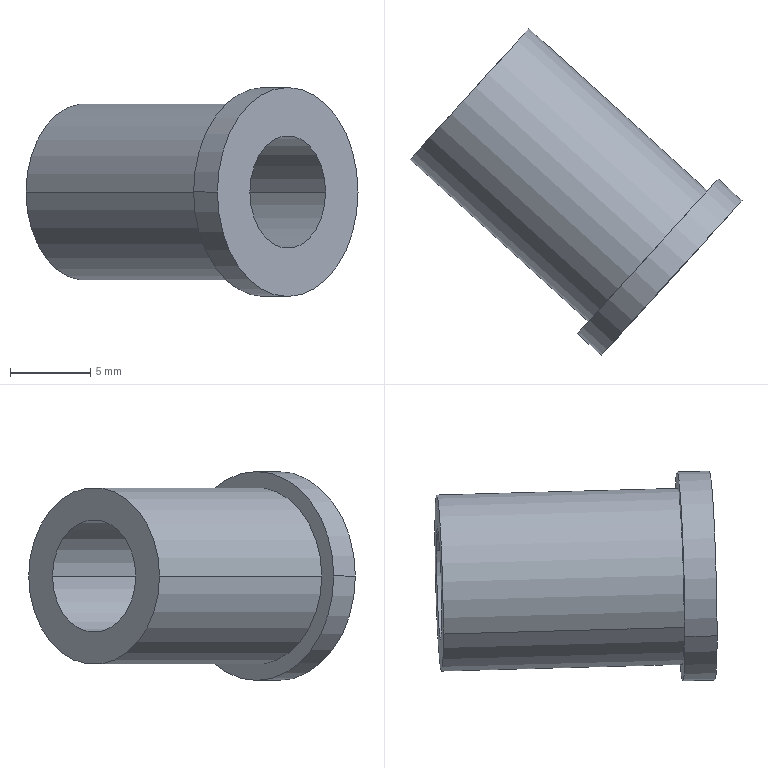Part | STEP file | PRT0001_68_29 | 1 solid | 9 faces | box 20.651 x 20.315 x 13 mm | volume 1037 mm3 | cylinder 6 | plane 3 | commonest cylinder face diameters 7 x2 11 x2 13 x2
STEP:
#1=CARTESIAN_POINT('',(0.,0.,0.));
#2=DIRECTION('',(0.,0.,1.));
#3=DIRECTION('',(1.,0.,0.));
#4=AXIS2_PLACEMENT_3D('',#1,#2,#3);
#5=CARTESIAN_POINT('',(1767.354,865.18,0.000000606));
#6=VERTEX_POINT('',#5);
#7=CARTESIAN_POINT('',(1774.754,873.318,0.000000606));
#8=VERTEX_POINT('',#7);
#9=CARTESIAN_POINT('',(1771.054,869.249,0.000000606));
#10=DIRECTION('',(0.7399,-0.6727,0.));
#11=DIRECTION('',(-0.6727,-0.7399,0.));
#12=AXIS2_PLACEMENT_3D('',#9,#10,#11);
#13=CIRCLE('',#12,5.5);
#14=CARTESIAN_POINT('',(536.884,-488.145,-24.));
#15=DIRECTION('',(-0.7399,0.6727,0.));
#16=DIRECTION('',(0.6727,0.7399,0.));
#17=AXIS2_PLACEMENT_3D('',#14,#15,#16);
#18=PLANE('',#17);
#19=CARTESIAN_POINT('',(1829.083,-24.));
#20=CARTESIAN_POINT('',(1829.083,-14.474));
#21=CARTESIAN_POINT('',(1837.333,-19.237));
#22=CARTESIAN_POINT('',(1845.583,-24.));
#23=CARTESIAN_POINT('',(1837.333,-28.763));
#24=CARTESIAN_POINT('',(1829.083,-33.526));
#25=CARTESIAN_POINT('',(1829.083,-24.));
#26=(BOUNDED_CURVE()B_SPLINE_CURVE(2,(#19,#20,#21,#22,#23,#24,#25),.UNSPECIFIED.,.T.,.F.)B_SPLINE_CURVE_WITH_KNOTS((1,2,2,2,2,1),(-2.094,0.,2.094,4.189,6.283,8.378),.UNSPECIFIED.)CURVE()GEOMETRIC_REPRESENTATION_ITEM()RATIONAL_B_SPLINE_CURVE((1.,0.5,1.,0.5,1.,0.5,1.))REPRESENTATION_ITEM(''));
#27=(GEOMETRIC_REPRESENTATION_CONTEXT(2)PARAMETRIC_REPRESENTATION_CONTEXT()REPRESENTATION_CONTEXT('',''));
#28=DEFINITIONAL_REPRESENTATION('',(#26),#27);
#29=PCURVE('',#18,#28);
#30=CARTESIAN_POINT('',(1780.673,860.504,0.000000606));
#31=DIRECTION('',(-0.7399,0.6727,0.));
#32=DIRECTION('',(0.6727,0.7399,0.));
#33=AXIS2_PLACEMENT_3D('',#30,#31,#32);
#34=CYLINDRICAL_SURFACE('',#33,5.5);
#35=CARTESIAN_POINT('',(3.142,13.));
#36=DIRECTION('',(-1.,0.));
#37=VECTOR('',#36,1.);
#38=LINE('',#35,#37);
#39=(GEOMETRIC_REPRESENTATION_CONTEXT(2)PARAMETRIC_REPRESENTATION_CONTEXT()REPRESENTATION_CONTEXT('',''));
#40=DEFINITIONAL_REPRESENTATION('',(#38),#39);
#41=PCURVE('',#34,#40);
#42=SURFACE_CURVE('',#13,(#29,#41),.PCURVE_S1.);
#43=EDGE_CURVE('',#6,#8,#42,.T.);
#44=ORIENTED_EDGE('',*,*,#43,.T.);
#45=CARTESIAN_POINT('',(1771.054,869.249,0.000000606));
#46=DIRECTION('',(0.7399,-0.6727,0.));
#47=DIRECTION('',(0.6727,0.7399,0.));
#48=AXIS2_PLACEMENT_3D('',#45,#46,#47);
#49=CIRCLE('',#48,5.5);
#50=CARTESIAN_POINT('',(1840.083,-24.));
#51=CARTESIAN_POINT('',(1840.083,-33.526));
#52=CARTESIAN_POINT('',(1831.833,-28.763));
#53=CARTESIAN_POINT('',(1823.583,-24.));
#54=CARTESIAN_POINT('',(1831.833,-19.237));
#55=CARTESIAN_POINT('',(1840.083,-14.474));
#56=CARTESIAN_POINT('',(1840.083,-24.));
#57=(BOUNDED_CURVE()B_SPLINE_CURVE(2,(#50,#51,#52,#53,#54,#55,#56),.UNSPECIFIED.,.T.,.F.)B_SPLINE_CURVE_WITH_KNOTS((1,2,2,2,2,1),(-2.094,0.,2.094,4.189,6.283,8.378),.UNSPECIFIED.)CURVE()GEOMETRIC_REPRESENTATION_ITEM()RATIONAL_B_SPLINE_CURVE((1.,0.5,1.,0.5,1.,0.5,1.))REPRESENTATION_ITEM(''));
#58=(GEOMETRIC_REPRESENTATION_CONTEXT(2)PARAMETRIC_REPRESENTATION_CONTEXT()REPRESENTATION_CONTEXT('',''));
#59=DEFINITIONAL_REPRESENTATION('',(#57),#58);
#60=PCURVE('',#18,#59);
#61=CARTESIAN_POINT('',(1780.673,860.504,0.000000606));
#62=DIRECTION('',(-0.7399,0.6727,0.));
#63=DIRECTION('',(0.6727,0.7399,0.));
#64=AXIS2_PLACEMENT_3D('',#61,#62,#63);
#65=CYLINDRICAL_SURFACE('',#64,5.5);
#66=CARTESIAN_POINT('',(6.283,13.));
#67=DIRECTION('',(-1.,0.));
#68=VECTOR('',#67,1.);
#69=LINE('',#66,#68);
#70=(GEOMETRIC_REPRESENTATION_CONTEXT(2)PARAMETRIC_REPRESENTATION_CONTEXT()REPRESENTATION_CONTEXT('',''));
#71=DEFINITIONAL_REPRESENTATION('',(#69),#70);
#72=PCURVE('',#65,#71);
#73=SURFACE_CURVE('',#49,(#60,#72),.PCURVE_S1.);
#74=EDGE_CURVE('',#8,#6,#73,.T.);
#75=ORIENTED_EDGE('',*,*,#74,.T.);
#76=EDGE_LOOP('',(#44,#75));
#77=FACE_BOUND('',#76,.F.);
#78=CARTESIAN_POINT('',(1768.7,866.659,0.000000606));
#79=VERTEX_POINT('',#78);
#80=CARTESIAN_POINT('',(1773.409,871.839,0.000000606));
#81=VERTEX_POINT('',#80);
#82=CARTESIAN_POINT('',(1771.054,869.249,0.000000606));
#83=DIRECTION('',(-0.7399,0.6727,0.));
#84=DIRECTION('',(-0.6727,-0.7399,0.));
#85=AXIS2_PLACEMENT_3D('',#82,#83,#84);
#86=CIRCLE('',#85,3.5);
#87=CARTESIAN_POINT('',(1834.583,-24.));
#88=DIRECTION('',(-1.,0.));
#89=AXIS2_PLACEMENT_2D('',#87,#88);
#90=CIRCLE('',#89,3.5);
#91=(GEOMETRIC_REPRESENTATION_CONTEXT(2)PARAMETRIC_REPRESENTATION_CONTEXT()REPRESENTATION_CONTEXT('',''));
#92=DEFINITIONAL_REPRESENTATION('',(#90),#91);
#93=PCURVE('',#18,#92);
#94=CARTESIAN_POINT('',(1780.673,860.504,0.000000606));
#95=DIRECTION('',(-0.7399,0.6727,0.));
#96=DIRECTION('',(0.6727,0.7399,0.));
#97=AXIS2_PLACEMENT_3D('',#94,#95,#96);
#98=CYLINDRICAL_SURFACE('',#97,3.5);
#99=CARTESIAN_POINT('',(3.142,13.));
#100=DIRECTION('',(1.,0.));
#101=VECTOR('',#100,1.);
#102=LINE('',#99,#101);
#103=(GEOMETRIC_REPRESENTATION_CONTEXT(2)PARAMETRIC_REPRESENTATION_CONTEXT()REPRESENTATION_CONTEXT('',''));
#104=DEFINITIONAL_REPRESENTATION('',(#102),#103);
#105=PCURVE('',#98,#104);
#106=SURFACE_CURVE('',#86,(#93,#105),.PCURVE_S1.);
#107=EDGE_CURVE('',#79,#81,#106,.T.);
#108=ORIENTED_EDGE('',*,*,#107,.T.);
#109=CARTESIAN_POINT('',(1771.054,869.249,0.000000606));
#110=DIRECTION('',(-0.7399,0.6727,0.));
#111=DIRECTION('',(0.6727,0.7399,0.));
#112=AXIS2_PLACEMENT_3D('',#109,#110,#111);
#113=CIRCLE('',#112,3.5);
#114=CARTESIAN_POINT('',(1834.583,-24.));
#115=DIRECTION('',(1.,0.));
#116=AXIS2_PLACEMENT_2D('',#114,#115);
#117=CIRCLE('',#116,3.5);
#118=(GEOMETRIC_REPRESENTATION_CONTEXT(2)PARAMETRIC_REPRESENTATION_CONTEXT()REPRESENTATION_CONTEXT('',''));
#119=DEFINITIONAL_REPRESENTATION('',(#117),#118);
#120=PCURVE('',#18,#119);
#121=CARTESIAN_POINT('',(1780.673,860.504,0.000000606));
#122=DIRECTION('',(-0.7399,0.6727,0.));
#123=DIRECTION('',(0.6727,0.7399,0.));
#124=AXIS2_PLACEMENT_3D('',#121,#122,#123);
#125=CYLINDRICAL_SURFACE('',#124,3.5);
#126=CARTESIAN_POINT('',(0.,13.));
#127=DIRECTION('',(1.,0.));
#128=VECTOR('',#127,1.);
#129=LINE('',#126,#128);
#130=(GEOMETRIC_REPRESENTATION_CONTEXT(2)PARAMETRIC_REPRESENTATION_CONTEXT()REPRESENTATION_CONTEXT('',''));
#131=DEFINITIONAL_REPRESENTATION('',(#129),#130);
#132=PCURVE('',#125,#131);
#133=SURFACE_CURVE('',#113,(#120,#132),.PCURVE_S1.);
#134=EDGE_CURVE('',#81,#79,#133,.T.);
#135=ORIENTED_EDGE('',*,*,#134,.T.);
#136=EDGE_LOOP('',(#108,#135));
#137=FACE_BOUND('',#136,.F.);
#138=ADVANCED_FACE('',(#77,#137),#18,.T.);
#139=CARTESIAN_POINT('',(1778.452,855.089,0.000000606));
#140=VERTEX_POINT('',#139);
#141=CARTESIAN_POINT('',(1767.354,865.18,0.000000606));
#142=DIRECTION('',(0.7399,-0.6727,0.));
#143=VECTOR('',#142,1.);
#144=LINE('',#141,#143);
#145=CARTESIAN_POINT('',(3.142,13.));
#146=DIRECTION('',(0.,-1.));
#147=VECTOR('',#146,1.);
#148=LINE('',#145,#147);
#149=(GEOMETRIC_REPRESENTATION_CONTEXT(2)PARAMETRIC_REPRESENTATION_CONTEXT()REPRESENTATION_CONTEXT('',''));
#150=DEFINITIONAL_REPRESENTATION('',(#148),#149);
#151=PCURVE('',#34,#150);
#152=CARTESIAN_POINT('',(3.142,13.));
#153=DIRECTION('',(0.,-1.));
#154=VECTOR('',#153,1.);
#155=LINE('',#152,#154);
#156=(GEOMETRIC_REPRESENTATION_CONTEXT(2)PARAMETRIC_REPRESENTATION_CONTEXT()REPRESENTATION_CONTEXT('',''));
#157=DEFINITIONAL_REPRESENTATION('',(#155),#156);
#158=PCURVE('',#65,#157);
#159=SURFACE_CURVE('',#144,(#151,#158),.PCURVE_S1.);
#160=EDGE_CURVE('',#6,#140,#159,.T.);
#161=ORIENTED_EDGE('',*,*,#160,.F.);
#162=ORIENTED_EDGE('',*,*,#43,.T.);
#163=CARTESIAN_POINT('',(1785.852,863.228,0.000000606));
#164=VERTEX_POINT('',#163);
#165=CARTESIAN_POINT('',(1774.754,873.318,0.000000606));
#166=DIRECTION('',(0.7399,-0.6727,0.));
#167=VECTOR('',#166,1.);
#168=LINE('',#165,#167);
#169=CARTESIAN_POINT('',(0.,13.));
#170=DIRECTION('',(0.,-1.));
#171=VECTOR('',#170,1.);
#172=LINE('',#169,#171);
#173=(GEOMETRIC_REPRESENTATION_CONTEXT(2)PARAMETRIC_REPRESENTATION_CONTEXT()REPRESENTATION_CONTEXT('',''));
#174=DEFINITIONAL_REPRESENTATION('',(#172),#173);
#175=PCURVE('',#34,#174);
#176=CARTESIAN_POINT('',(6.283,13.));
#177=DIRECTION('',(0.,-1.));
#178=VECTOR('',#177,1.);
#179=LINE('',#176,#178);
#180=(GEOMETRIC_REPRESENTATION_CONTEXT(2)PARAMETRIC_REPRESENTATION_CONTEXT()REPRESENTATION_CONTEXT('',''));
#181=DEFINITIONAL_REPRESENTATION('',(#179),#180);
#182=PCURVE('',#65,#181);
#183=SURFACE_CURVE('',#168,(#175,#182),.PCURVE_S1.);
#184=EDGE_CURVE('',#8,#164,#183,.T.);
#185=ORIENTED_EDGE('',*,*,#184,.T.);
#186=CARTESIAN_POINT('',(1782.152,859.158,0.000000606));
#187=DIRECTION('',(-0.7399,0.6727,0.));
#188=DIRECTION('',(0.6727,0.7399,0.));
#189=AXIS2_PLACEMENT_3D('',#186,#187,#188);
#190=CIRCLE('',#189,5.5);
#191=CARTESIAN_POINT('',(0.,-2.));
#192=DIRECTION('',(1.,0.));
#193=VECTOR('',#192,1.);
#194=LINE('',#191,#193);
#195=(GEOMETRIC_REPRESENTATION_CONTEXT(2)PARAMETRIC_REPRESENTATION_CONTEXT()REPRESENTATION_CONTEXT('',''));
#196=DEFINITIONAL_REPRESENTATION('',(#194),#195);
#197=PCURVE('',#34,#196);
#198=CARTESIAN_POINT('',(547.982,-498.236,0.));
#199=DIRECTION('',(0.7399,-0.6727,0.));
#200=DIRECTION('',(0.6727,0.7399,0.));
#201=AXIS2_PLACEMENT_3D('',#198,#199,#200);
#202=PLANE('',#201);
#203=CARTESIAN_POINT('',(1840.083,0.000000606));
#204=CARTESIAN_POINT('',(1840.083,-9.526));
#205=CARTESIAN_POINT('',(1831.833,-4.763));
#206=CARTESIAN_POINT('',(1823.583,0.000000606));
#207=CARTESIAN_POINT('',(1831.833,4.763));
#208=CARTESIAN_POINT('',(1840.083,9.526));
#209=CARTESIAN_POINT('',(1840.083,0.000000606));
#210=(BOUNDED_CURVE()B_SPLINE_CURVE(2,(#203,#204,#205,#206,#207,#208,#209),.UNSPECIFIED.,.T.,.F.)B_SPLINE_CURVE_WITH_KNOTS((1,2,2,2,2,1),(-2.094,0.,2.094,4.189,6.283,8.378),.UNSPECIFIED.)CURVE()GEOMETRIC_REPRESENTATION_ITEM()RATIONAL_B_SPLINE_CURVE((1.,0.5,1.,0.5,1.,0.5,1.))REPRESENTATION_ITEM(''));
#211=(GEOMETRIC_REPRESENTATION_CONTEXT(2)PARAMETRIC_REPRESENTATION_CONTEXT()REPRESENTATION_CONTEXT('',''));
#212=DEFINITIONAL_REPRESENTATION('',(#210),#211);
#213=PCURVE('',#202,#212);
#214=SURFACE_CURVE('',#190,(#197,#213),.PCURVE_S1.);
#215=EDGE_CURVE('',#164,#140,#214,.T.);
#216=ORIENTED_EDGE('',*,*,#215,.T.);
#217=EDGE_LOOP('',(#161,#162,#185,#216));
#218=FACE_BOUND('',#217,.T.);
#219=ADVANCED_FACE('',(#218),#34,.T.);
#220=CARTESIAN_POINT('',(1786.525,863.967,0.000000606));
#221=VERTEX_POINT('',#220);
#222=CARTESIAN_POINT('',(1777.78,854.349,0.000000606));
#223=VERTEX_POINT('',#222);
#224=CARTESIAN_POINT('',(1782.152,859.158,0.000000606));
#225=DIRECTION('',(0.7399,-0.6727,0.));
#226=DIRECTION('',(0.6727,0.7399,0.));
#227=AXIS2_PLACEMENT_3D('',#224,#225,#226);
#228=CIRCLE('',#227,6.5);
#229=CARTESIAN_POINT('',(1834.583,0.000000606));
#230=DIRECTION('',(1.,0.));
#231=AXIS2_PLACEMENT_2D('',#229,#230);
#232=CIRCLE('',#231,6.5);
#233=(GEOMETRIC_REPRESENTATION_CONTEXT(2)PARAMETRIC_REPRESENTATION_CONTEXT()REPRESENTATION_CONTEXT('',''));
#234=DEFINITIONAL_REPRESENTATION('',(#232),#233);
#235=PCURVE('',#202,#234);
#236=CARTESIAN_POINT('',(1782.152,859.158,0.000000606));
#237=DIRECTION('',(0.7399,-0.6727,0.));
#238=DIRECTION('',(0.6727,0.7399,0.));
#239=AXIS2_PLACEMENT_3D('',#236,#237,#238);
#240=CYLINDRICAL_SURFACE('',#239,6.5);
#241=CARTESIAN_POINT('',(0.,0.));
#242=DIRECTION('',(1.,0.));
#243=VECTOR('',#242,1.);
#244=LINE('',#241,#243);
#245=(GEOMETRIC_REPRESENTATION_CONTEXT(2)PARAMETRIC_REPRESENTATION_CONTEXT()REPRESENTATION_CONTEXT('',''));
#246=DEFINITIONAL_REPRESENTATION('',(#244),#245);
#247=PCURVE('',#240,#246);
#248=SURFACE_CURVE('',#228,(#235,#247),.PCURVE_S1.);
#249=EDGE_CURVE('',#221,#223,#248,.T.);
#250=ORIENTED_EDGE('',*,*,#249,.T.);
#251=CARTESIAN_POINT('',(1782.152,859.158,0.000000606));
#252=DIRECTION('',(0.7399,-0.6727,0.));
#253=DIRECTION('',(-0.6727,-0.7399,0.));
#254=AXIS2_PLACEMENT_3D('',#251,#252,#253);
#255=CIRCLE('',#254,6.5);
#256=CARTESIAN_POINT('',(1834.583,0.000000606));
#257=DIRECTION('',(-1.,0.));
#258=AXIS2_PLACEMENT_2D('',#256,#257);
#259=CIRCLE('',#258,6.5);
#260=(GEOMETRIC_REPRESENTATION_CONTEXT(2)PARAMETRIC_REPRESENTATION_CONTEXT()REPRESENTATION_CONTEXT('',''));
#261=DEFINITIONAL_REPRESENTATION('',(#259),#260);
#262=PCURVE('',#202,#261);
#263=CARTESIAN_POINT('',(1782.152,859.158,0.000000606));
#264=DIRECTION('',(0.7399,-0.6727,0.));
#265=DIRECTION('',(0.6727,0.7399,0.));
#266=AXIS2_PLACEMENT_3D('',#263,#264,#265);
#267=CYLINDRICAL_SURFACE('',#266,6.5);
#268=CARTESIAN_POINT('',(3.142,0.));
#269=DIRECTION('',(1.,0.));
#270=VECTOR('',#269,1.);
#271=LINE('',#268,#270);
#272=(GEOMETRIC_REPRESENTATION_CONTEXT(2)PARAMETRIC_REPRESENTATION_CONTEXT()REPRESENTATION_CONTEXT('',''));
#273=DEFINITIONAL_REPRESENTATION('',(#271),#272);
#274=PCURVE('',#267,#273);
#275=SURFACE_CURVE('',#255,(#262,#274),.PCURVE_S1.);
#276=EDGE_CURVE('',#223,#221,#275,.T.);
#277=ORIENTED_EDGE('',*,*,#276,.T.);
#278=EDGE_LOOP('',(#250,#277));
#279=FACE_BOUND('',#278,.F.);
#280=ORIENTED_EDGE('',*,*,#215,.T.);
#281=CARTESIAN_POINT('',(1782.152,859.158,0.000000606));
#282=DIRECTION('',(-0.7399,0.6727,0.));
#283=DIRECTION('',(-0.6727,-0.7399,0.));
#284=AXIS2_PLACEMENT_3D('',#281,#282,#283);
#285=CIRCLE('',#284,5.5);
#286=CARTESIAN_POINT('',(1829.083,0.000000606));
#287=CARTESIAN_POINT('',(1829.083,9.526));
#288=CARTESIAN_POINT('',(1837.333,4.763));
#289=CARTESIAN_POINT('',(1845.583,0.000000606));
#290=CARTESIAN_POINT('',(1837.333,-4.763));
#291=CARTESIAN_POINT('',(1829.083,-9.526));
#292=CARTESIAN_POINT('',(1829.083,0.000000606));
#293=(BOUNDED_CURVE()B_SPLINE_CURVE(2,(#286,#287,#288,#289,#290,#291,#292),.UNSPECIFIED.,.T.,.F.)B_SPLINE_CURVE_WITH_KNOTS((1,2,2,2,2,1),(-2.094,0.,2.094,4.189,6.283,8.378),.UNSPECIFIED.)CURVE()GEOMETRIC_REPRESENTATION_ITEM()RATIONAL_B_SPLINE_CURVE((1.,0.5,1.,0.5,1.,0.5,1.))REPRESENTATION_ITEM(''));
#294=(GEOMETRIC_REPRESENTATION_CONTEXT(2)PARAMETRIC_REPRESENTATION_CONTEXT()REPRESENTATION_CONTEXT('',''));
#295=DEFINITIONAL_REPRESENTATION('',(#293),#294);
#296=PCURVE('',#202,#295);
#297=CARTESIAN_POINT('',(3.142,-2.));
#298=DIRECTION('',(1.,0.));
#299=VECTOR('',#298,1.);
#300=LINE('',#297,#299);
#301=(GEOMETRIC_REPRESENTATION_CONTEXT(2)PARAMETRIC_REPRESENTATION_CONTEXT()REPRESENTATION_CONTEXT('',''));
#302=DEFINITIONAL_REPRESENTATION('',(#300),#301);
#303=PCURVE('',#65,#302);
#304=SURFACE_CURVE('',#285,(#296,#303),.PCURVE_S1.);
#305=EDGE_CURVE('',#140,#164,#304,.T.);
#306=ORIENTED_EDGE('',*,*,#305,.T.);
#307=EDGE_LOOP('',(#280,#306));
#308=FACE_BOUND('',#307,.F.);
#309=ADVANCED_FACE('',(#279,#308),#202,.F.);
#310=CARTESIAN_POINT('',(1779.26,853.003,0.000000606));
#311=VERTEX_POINT('',#310);
#312=CARTESIAN_POINT('',(1779.26,853.003,0.000000606));
#313=DIRECTION('',(-0.7399,0.6727,0.));
#314=VECTOR('',#313,1.);
#315=LINE('',#312,#314);
#316=CARTESIAN_POINT('',(3.142,2.));
#317=DIRECTION('',(0.,-1.));
#318=VECTOR('',#317,1.);
#319=LINE('',#316,#318);
#320=(GEOMETRIC_REPRESENTATION_CONTEXT(2)PARAMETRIC_REPRESENTATION_CONTEXT()REPRESENTATION_CONTEXT('',''));
#321=DEFINITIONAL_REPRESENTATION('',(#319),#320);
#322=PCURVE('',#240,#321);
#323=CARTESIAN_POINT('',(3.142,2.));
#324=DIRECTION('',(0.,-1.));
#325=VECTOR('',#324,1.);
#326=LINE('',#323,#325);
#327=(GEOMETRIC_REPRESENTATION_CONTEXT(2)PARAMETRIC_REPRESENTATION_CONTEXT()REPRESENTATION_CONTEXT('',''));
#328=DEFINITIONAL_REPRESENTATION('',(#326),#327);
#329=PCURVE('',#267,#328);
#330=SURFACE_CURVE('',#315,(#322,#329),.PCURVE_S1.);
#331=EDGE_CURVE('',#311,#223,#330,.T.);
#332=ORIENTED_EDGE('',*,*,#331,.F.);
#333=CARTESIAN_POINT('',(1788.005,862.622,0.000000606));
#334=VERTEX_POINT('',#333);
#335=CARTESIAN_POINT('',(1783.632,857.813,0.000000606));
#336=DIRECTION('',(-0.7399,0.6727,0.));
#337=DIRECTION('',(-0.6727,-0.7399,0.));
#338=AXIS2_PLACEMENT_3D('',#335,#336,#337);
#339=CIRCLE('',#338,6.5);
#340=CARTESIAN_POINT('',(3.142,2.));
#341=DIRECTION('',(-1.,0.));
#342=VECTOR('',#341,1.);
#343=LINE('',#340,#342);
#344=(GEOMETRIC_REPRESENTATION_CONTEXT(2)PARAMETRIC_REPRESENTATION_CONTEXT()REPRESENTATION_CONTEXT('',''));
#345=DEFINITIONAL_REPRESENTATION('',(#343),#344);
#346=PCURVE('',#240,#345);
#347=CARTESIAN_POINT('',(549.462,-499.582,0.));
#348=DIRECTION('',(0.7399,-0.6727,0.));
#349=DIRECTION('',(0.6727,0.7399,0.));
#350=AXIS2_PLACEMENT_3D('',#347,#348,#349);
#351=PLANE('',#350);
#352=CARTESIAN_POINT('',(1828.083,0.000000606));
#353=CARTESIAN_POINT('',(1828.083,11.258));
#354=CARTESIAN_POINT('',(1837.833,5.629));
#355=CARTESIAN_POINT('',(1847.583,0.000000606));
#356=CARTESIAN_POINT('',(1837.833,-5.629));
#357=CARTESIAN_POINT('',(1828.083,-11.258));
#358=CARTESIAN_POINT('',(1828.083,0.000000606));
#359=(BOUNDED_CURVE()B_SPLINE_CURVE(2,(#352,#353,#354,#355,#356,#357,#358),.UNSPECIFIED.,.T.,.F.)B_SPLINE_CURVE_WITH_KNOTS((1,2,2,2,2,1),(-2.094,0.,2.094,4.189,6.283,8.378),.UNSPECIFIED.)CURVE()GEOMETRIC_REPRESENTATION_ITEM()RATIONAL_B_SPLINE_CURVE((1.,0.5,1.,0.5,1.,0.5,1.))REPRESENTATION_ITEM(''));
#360=(GEOMETRIC_REPRESENTATION_CONTEXT(2)PARAMETRIC_REPRESENTATION_CONTEXT()REPRESENTATION_CONTEXT('',''));
#361=DEFINITIONAL_REPRESENTATION('',(#359),#360);
#362=PCURVE('',#351,#361);
#363=SURFACE_CURVE('',#339,(#346,#362),.PCURVE_S1.);
#364=EDGE_CURVE('',#311,#334,#363,.T.);
#365=ORIENTED_EDGE('',*,*,#364,.T.);
#366=CARTESIAN_POINT('',(1788.005,862.622,0.000000606));
#367=DIRECTION('',(-0.7399,0.6727,0.));
#368=VECTOR('',#367,1.);
#369=LINE('',#366,#368);
#370=CARTESIAN_POINT('',(0.,2.));
#371=DIRECTION('',(0.,-1.));
#372=VECTOR('',#371,1.);
#373=LINE('',#370,#372);
#374=(GEOMETRIC_REPRESENTATION_CONTEXT(2)PARAMETRIC_REPRESENTATION_CONTEXT()REPRESENTATION_CONTEXT('',''));
#375=DEFINITIONAL_REPRESENTATION('',(#373),#374);
#376=PCURVE('',#240,#375);
#377=CARTESIAN_POINT('',(6.283,2.));
#378=DIRECTION('',(0.,-1.));
#379=VECTOR('',#378,1.);
#380=LINE('',#377,#379);
#381=(GEOMETRIC_REPRESENTATION_CONTEXT(2)PARAMETRIC_REPRESENTATION_CONTEXT()REPRESENTATION_CONTEXT('',''));
#382=DEFINITIONAL_REPRESENTATION('',(#380),#381);
#383=PCURVE('',#267,#382);
#384=SURFACE_CURVE('',#369,(#376,#383),.PCURVE_S1.);
#385=EDGE_CURVE('',#334,#221,#384,.T.);
#386=ORIENTED_EDGE('',*,*,#385,.T.);
#387=ORIENTED_EDGE('',*,*,#249,.T.);
#388=EDGE_LOOP('',(#332,#365,#386,#387));
#389=FACE_BOUND('',#388,.T.);
#390=ADVANCED_FACE('',(#389),#240,.T.);
#391=ORIENTED_EDGE('',*,*,#385,.F.);
#392=CARTESIAN_POINT('',(1783.632,857.813,0.000000606));
#393=DIRECTION('',(-0.7399,0.6727,0.));
#394=DIRECTION('',(0.6727,0.7399,0.));
#395=AXIS2_PLACEMENT_3D('',#392,#393,#394);
#396=CIRCLE('',#395,6.5);
#397=CARTESIAN_POINT('',(6.283,2.));
#398=DIRECTION('',(-1.,0.));
#399=VECTOR('',#398,1.);
#400=LINE('',#397,#399);
#401=(GEOMETRIC_REPRESENTATION_CONTEXT(2)PARAMETRIC_REPRESENTATION_CONTEXT()REPRESENTATION_CONTEXT('',''));
#402=DEFINITIONAL_REPRESENTATION('',(#400),#401);
#403=PCURVE('',#267,#402);
#404=CARTESIAN_POINT('',(1841.083,0.000000606));
#405=CARTESIAN_POINT('',(1841.083,-11.258));
#406=CARTESIAN_POINT('',(1831.333,-5.629));
#407=CARTESIAN_POINT('',(1821.583,0.000000606));
#408=CARTESIAN_POINT('',(1831.333,5.629));
#409=CARTESIAN_POINT('',(1841.083,11.258));
#410=CARTESIAN_POINT('',(1841.083,0.000000606));
#411=(BOUNDED_CURVE()B_SPLINE_CURVE(2,(#404,#405,#406,#407,#408,#409,#410),.UNSPECIFIED.,.T.,.F.)B_SPLINE_CURVE_WITH_KNOTS((1,2,2,2,2,1),(-2.094,0.,2.094,4.189,6.283,8.378),.UNSPECIFIED.)CURVE()GEOMETRIC_REPRESENTATION_ITEM()RATIONAL_B_SPLINE_CURVE((1.,0.5,1.,0.5,1.,0.5,1.))REPRESENTATION_ITEM(''));
#412=(GEOMETRIC_REPRESENTATION_CONTEXT(2)PARAMETRIC_REPRESENTATION_CONTEXT()REPRESENTATION_CONTEXT('',''));
#413=DEFINITIONAL_REPRESENTATION('',(#411),#412);
#414=PCURVE('',#351,#413);
#415=SURFACE_CURVE('',#396,(#403,#414),.PCURVE_S1.);
#416=EDGE_CURVE('',#334,#311,#415,.T.);
#417=ORIENTED_EDGE('',*,*,#416,.T.);
#418=ORIENTED_EDGE('',*,*,#331,.T.);
#419=ORIENTED_EDGE('',*,*,#276,.T.);
#420=EDGE_LOOP('',(#391,#417,#418,#419));
#421=FACE_BOUND('',#420,.T.);
#422=ADVANCED_FACE('',(#421),#267,.T.);
#423=ORIENTED_EDGE('',*,*,#364,.T.);
#424=ORIENTED_EDGE('',*,*,#416,.T.);
#425=EDGE_LOOP('',(#423,#424));
#426=FACE_BOUND('',#425,.F.);
#427=CARTESIAN_POINT('',(1781.278,855.223,0.000000606));
#428=VERTEX_POINT('',#427);
#429=CARTESIAN_POINT('',(1785.987,860.402,0.000000606));
#430=VERTEX_POINT('',#429);
#431=CARTESIAN_POINT('',(1783.632,857.813,0.000000606));
#432=DIRECTION('',(0.7399,-0.6727,0.));
#433=DIRECTION('',(-0.6727,-0.7399,0.));
#434=AXIS2_PLACEMENT_3D('',#431,#432,#433);
#435=CIRCLE('',#434,3.5);
#436=CARTESIAN_POINT('',(1834.583,0.000000606));
#437=DIRECTION('',(-1.,0.));
#438=AXIS2_PLACEMENT_2D('',#436,#437);
#439=CIRCLE('',#438,3.5);
#440=(GEOMETRIC_REPRESENTATION_CONTEXT(2)PARAMETRIC_REPRESENTATION_CONTEXT()REPRESENTATION_CONTEXT('',''));
#441=DEFINITIONAL_REPRESENTATION('',(#439),#440);
#442=PCURVE('',#351,#441);
#443=CARTESIAN_POINT('',(3.142,-4.));
#444=DIRECTION('',(-1.,0.));
#445=VECTOR('',#444,1.);
#446=LINE('',#443,#445);
#447=(GEOMETRIC_REPRESENTATION_CONTEXT(2)PARAMETRIC_REPRESENTATION_CONTEXT()REPRESENTATION_CONTEXT('',''));
#448=DEFINITIONAL_REPRESENTATION('',(#446),#447);
#449=PCURVE('',#125,#448);
#450=SURFACE_CURVE('',#435,(#442,#449),.PCURVE_S1.);
#451=EDGE_CURVE('',#428,#430,#450,.T.);
#452=ORIENTED_EDGE('',*,*,#451,.T.);
#453=CARTESIAN_POINT('',(1783.632,857.813,0.000000606));
#454=DIRECTION('',(0.7399,-0.6727,0.));
#455=DIRECTION('',(0.6727,0.7399,0.));
#456=AXIS2_PLACEMENT_3D('',#453,#454,#455);
#457=CIRCLE('',#456,3.5);
#458=CARTESIAN_POINT('',(1834.583,0.000000606));
#459=DIRECTION('',(1.,0.));
#460=AXIS2_PLACEMENT_2D('',#458,#459);
#461=CIRCLE('',#460,3.5);
#462=(GEOMETRIC_REPRESENTATION_CONTEXT(2)PARAMETRIC_REPRESENTATION_CONTEXT()REPRESENTATION_CONTEXT('',''));
#463=DEFINITIONAL_REPRESENTATION('',(#461),#462);
#464=PCURVE('',#351,#463);
#465=CARTESIAN_POINT('',(6.283,-4.));
#466=DIRECTION('',(-1.,0.));
#467=VECTOR('',#466,1.);
#468=LINE('',#465,#467);
#469=(GEOMETRIC_REPRESENTATION_CONTEXT(2)PARAMETRIC_REPRESENTATION_CONTEXT()REPRESENTATION_CONTEXT('',''));
#470=DEFINITIONAL_REPRESENTATION('',(#468),#469);
#471=PCURVE('',#98,#470);
#472=SURFACE_CURVE('',#457,(#464,#471),.PCURVE_S1.);
#473=EDGE_CURVE('',#430,#428,#472,.T.);
#474=ORIENTED_EDGE('',*,*,#473,.T.);
#475=EDGE_LOOP('',(#452,#474));
#476=FACE_BOUND('',#475,.F.);
#477=ADVANCED_FACE('',(#426,#476),#351,.T.);
#478=CARTESIAN_POINT('',(1773.409,871.839,0.000000606));
#479=DIRECTION('',(0.7399,-0.6727,0.));
#480=VECTOR('',#479,1.);
#481=LINE('',#478,#480);
#482=CARTESIAN_POINT('',(0.,13.));
#483=DIRECTION('',(0.,-1.));
#484=VECTOR('',#483,1.);
#485=LINE('',#482,#484);
#486=(GEOMETRIC_REPRESENTATION_CONTEXT(2)PARAMETRIC_REPRESENTATION_CONTEXT()REPRESENTATION_CONTEXT('',''));
#487=DEFINITIONAL_REPRESENTATION('',(#485),#486);
#488=PCURVE('',#125,#487);
#489=CARTESIAN_POINT('',(6.283,13.));
#490=DIRECTION('',(0.,-1.));
#491=VECTOR('',#490,1.);
#492=LINE('',#489,#491);
#493=(GEOMETRIC_REPRESENTATION_CONTEXT(2)PARAMETRIC_REPRESENTATION_CONTEXT()REPRESENTATION_CONTEXT('',''));
#494=DEFINITIONAL_REPRESENTATION('',(#492),#493);
#495=PCURVE('',#98,#494);
#496=SURFACE_CURVE('',#481,(#488,#495),.PCURVE_S1.);
#497=EDGE_CURVE('',#81,#430,#496,.T.);
#498=ORIENTED_EDGE('',*,*,#497,.T.);
#499=ORIENTED_EDGE('',*,*,#451,.F.);
#500=CARTESIAN_POINT('',(1781.278,855.223,0.000000606));
#501=DIRECTION('',(-0.7399,0.6727,0.));
#502=VECTOR('',#501,1.);
#503=LINE('',#500,#502);
#504=CARTESIAN_POINT('',(3.142,-4.));
#505=DIRECTION('',(0.,1.));
#506=VECTOR('',#505,1.);
#507=LINE('',#504,#506);
#508=(GEOMETRIC_REPRESENTATION_CONTEXT(2)PARAMETRIC_REPRESENTATION_CONTEXT()REPRESENTATION_CONTEXT('',''));
#509=DEFINITIONAL_REPRESENTATION('',(#507),#508);
#510=PCURVE('',#125,#509);
#511=CARTESIAN_POINT('',(3.142,-4.));
#512=DIRECTION('',(0.,1.));
#513=VECTOR('',#512,1.);
#514=LINE('',#511,#513);
#515=(GEOMETRIC_REPRESENTATION_CONTEXT(2)PARAMETRIC_REPRESENTATION_CONTEXT()REPRESENTATION_CONTEXT('',''));
#516=DEFINITIONAL_REPRESENTATION('',(#514),#515);
#517=PCURVE('',#98,#516);
#518=SURFACE_CURVE('',#503,(#510,#517),.PCURVE_S1.);
#519=EDGE_CURVE('',#428,#79,#518,.T.);
#520=ORIENTED_EDGE('',*,*,#519,.T.);
#521=ORIENTED_EDGE('',*,*,#134,.F.);
#522=EDGE_LOOP('',(#498,#499,#520,#521));
#523=FACE_BOUND('',#522,.F.);
#524=ADVANCED_FACE('',(#523),#125,.F.);
#525=ORIENTED_EDGE('',*,*,#519,.F.);
#526=ORIENTED_EDGE('',*,*,#473,.F.);
#527=ORIENTED_EDGE('',*,*,#497,.F.);
#528=ORIENTED_EDGE('',*,*,#107,.F.);
#529=EDGE_LOOP('',(#525,#526,#527,#528));
#530=FACE_BOUND('',#529,.F.);
#531=ADVANCED_FACE('',(#530),#98,.F.);
#532=ORIENTED_EDGE('',*,*,#184,.F.);
#533=ORIENTED_EDGE('',*,*,#74,.T.);
#534=ORIENTED_EDGE('',*,*,#160,.T.);
#535=ORIENTED_EDGE('',*,*,#305,.T.);
#536=EDGE_LOOP('',(#532,#533,#534,#535));
#537=FACE_BOUND('',#536,.T.);
#538=ADVANCED_FACE('',(#537),#65,.T.);
#539=CLOSED_SHELL('',(#138,#219,#309,#390,#422,#477,#524,#531,#538));
#540=MANIFOLD_SOLID_BREP('',#539);
#541=(LENGTH_UNIT()NAMED_UNIT(*)SI_UNIT(.MILLI.,.METRE.));
#542=UNCERTAINTY_MEASURE_WITH_UNIT(LENGTH_MEASURE(0.0000001),#541,'','');
#543=(NAMED_UNIT(*)PLANE_ANGLE_UNIT()SI_UNIT($,.RADIAN.));
#544=(NAMED_UNIT(*)SI_UNIT($,.STERADIAN.)SOLID_ANGLE_UNIT());
#545=(GEOMETRIC_REPRESENTATION_CONTEXT(3)GLOBAL_UNCERTAINTY_ASSIGNED_CONTEXT((#542))GLOBAL_UNIT_ASSIGNED_CONTEXT((#541,#543,#544))REPRESENTATION_CONTEXT('',''));
#546=ADVANCED_BREP_SHAPE_REPRESENTATION('',(#4,#540),#545);